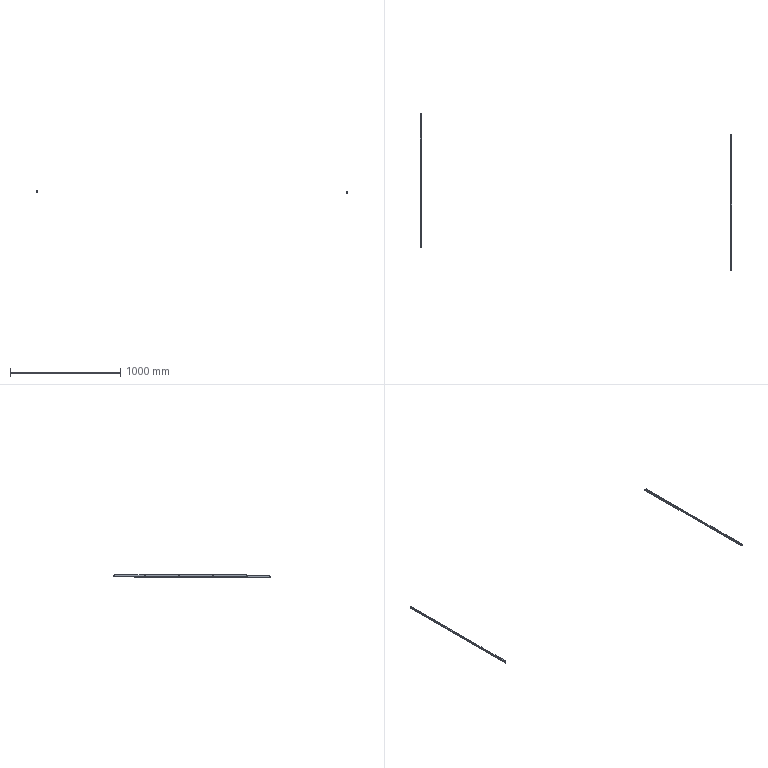NC program | NX | posted with a generic post | part box 2829 x 1430 x 20 mm
Whole program:
N10 G17 G21 G94 G90
(PLANAR_MILL_COPY_COPY_1 , TOOL : D16-48-D16-100-3T-FINISH)
N12 T01 M6
N14 G54
N16 G17 G0 G90 X623.5 Y0. B0. C0. S4000 M3
N18 G43 Z34. H1
N20 Z5.
N22 G94 G1 Z3. F1000.
N24 X610.5
N26 X-610.5
N28 X-623.5
N30 Z5.
N32 G0 Z34.
N34 X623.5
N36 Z4.
N38 G1 Z2.
N40 X610.5
N42 X-610.5
N44 X-623.5
N46 Z4.
N48 G0 Z34.
N50 X623.5
N52 Z3.
N54 G1 Z1.
N56 X610.5
N58 X-610.5
N60 X-623.5
N62 Z3.
N64 G0 Z34.
N66 X623.5
N68 Z2.1
N70 G1 Z0.1
N72 X610.5
N74 X-610.5
N76 X-623.5
N78 Z2.1
N80 G0 Z34.
(PLANAR_MILL_COPY_COPY_1_COPY , TOOL : D16-48-D16-100-3T-FINISH)
N82 X623.5
N84 Z2.
N86 G1 Z0.
N88 X610.5
N90 X-610.5
N92 X-623.5
N94 Z2.
N96 G0 Z34.
N98 M5
(PLANAR_MILL_2_COPY_1 , TOOL : D8-25-D8-60-3T-FINISH)
N100 T03 M6
N102 G54
N104 G17 G0 G90 X-606.4 Y11. B0. C0. S4500 M3
N106 G43 Z30. H3
N108 Z1.
N110 G94 G1 Z-1. F1200.
N112 Y5.
N114 Y-5.
N116 X-604.6
N118 Y5.
N120 Y11.
N122 Z1.
N124 G0 X-606.4 Z0.
N126 G1 Z-2.
N128 Y5.
N130 Y-5.
N132 X-604.6
N134 Y5.
N136 Y11.
N138 Z0.
N140 G0 X-606.4 Z-1.
N142 G1 Z-3.
N144 Y5.
N146 Y-5.
N148 X-604.6
N150 Y5.
N152 Y11.
N154 Z-1.
N156 G0 X-606.4 Z-2.
N158 G1 Z-4.
N160 Y5.
N162 Y-5.
N164 X-604.6
N166 Y5.
N168 Y11.
N170 Z-2.
N172 G0 X-606.4 Z-3.
N174 G1 Z-5.
N176 Y5.
N178 Y-5.
N180 X-604.6
N182 Y5.
N184 Y11.
N186 Z-3.
N188 G0 X-606.4 Z-4.
N190 G1 Z-6.
N192 Y5.
N194 Y-5.
N196 X-604.6
N198 Y5.
N200 Y11.
N202 Z-4.
N204 G0 X-606.4 Z-5.
N206 G1 Z-7.
N208 Y5.
N210 Y-5.
N212 X-604.6
N214 Y5.
N216 Y11.
N218 Z-5.
N220 G0 X-606.4 Z-5.9
N222 G1 Z-7.9
N224 Y5.
N226 Y-5.
N228 X-604.6
N230 Y5.
N232 Y11.
N234 Z-5.9
N236 G0 Z30.
N238 X-325.4
N240 Z1.
N242 G1 Z-1.
N244 Y5.
N246 Y-5.
N248 X-323.6
N250 Y5.
N252 Y11.
N254 Z1.
N256 G0 X-325.4 Z0.
N258 G1 Z-2.
N260 Y5.
N262 Y-5.
N264 X-323.6
N266 Y5.
N268 Y11.
N270 Z0.
N272 G0 X-325.4 Z-1.
N274 G1 Z-3.
N276 Y5.
N278 Y-5.
N280 X-323.6
N282 Y5.
N284 Y11.
N286 Z-1.
N288 G0 X-325.4 Z-2.
N290 G1 Z-4.
N292 Y5.
N294 Y-5.
N296 X-323.6
N298 Y5.
N300 Y11.
N302 Z-2.
N304 G0 X-325.4 Z-3.
N306 G1 Z-5.
N308 Y5.
N310 Y-5.
N312 X-323.6
N314 Y5.
N316 Y11.
N318 Z-3.
N320 G0 X-325.4 Z-4.
N322 G1 Z-6.
N324 Y5.
N326 Y-5.
N328 X-323.6
N330 Y5.
N332 Y11.
N334 Z-4.
N336 G0 X-325.4 Z-5.
N338 G1 Z-7.
N340 Y5.
N342 Y-5.
N344 X-323.6
N346 Y5.
N348 Y11.
N350 Z-5.
N352 G0 X-325.4 Z-5.9
N354 G1 Z-7.9
N356 Y5.
N358 Y-5.
N360 X-323.6
N362 Y5.
N364 Y11.
N366 Z-5.9
N368 G0 Z30.
N370 X-15.4
N372 Z1.
N374 G1 Z-1.
N376 Y5.
N378 Y-5.
N380 X-13.6
N382 Y5.
N384 Y11.
N386 Z1.
N388 G0 X-15.4 Z0.
N390 G1 Z-2.
N392 Y5.
N394 Y-5.
N396 X-13.6
N398 Y5.
N400 Y11.
N402 Z0.
N404 G0 X-15.4 Z-1.
N406 G1 Z-3.
N408 Y5.
N410 Y-5.
N412 X-13.6
N414 Y5.
N416 Y11.
N418 Z-1.
N420 G0 X-15.4 Z-2.
N422 G1 Z-4.
N424 Y5.
N426 Y-5.
N428 X-13.6
N430 Y5.
N432 Y11.
N434 Z-2.
N436 G0 X-15.4 Z-3.
N438 G1 Z-5.
N440 Y5.
N442 Y-5.
N444 X-13.6
N446 Y5.
N448 Y11.
N450 Z-3.
N452 G0 X-15.4 Z-4.
N454 G1 Z-6.
N456 Y5.
N458 Y-5.
N460 X-13.6
N462 Y5.
N464 Y11.
N466 Z-4.
N468 G0 X-15.4 Z-5.
N470 G1 Z-7.
N472 Y5.
N474 Y-5.
N476 X-13.6
N478 Y5.
N480 Y11.
N482 Z-5.
N484 G0 X-15.4 Z-5.9
N486 G1 Z-7.9
N488 Y5.
N490 Y-5.
N492 X-13.6
N494 Y5.
N496 Y11.
N498 Z-5.9
N500 G0 Z30.
N502 X294.6
N504 Z1.
N506 G1 Z-1.
N508 Y5.
N510 Y-5.
N512 X296.4
N514 Y5.
N516 Y11.
N518 Z1.
N520 G0 X294.6 Z0.
N522 G1 Z-2.
N524 Y5.
N526 Y-5.
N528 X296.4
N530 Y5.
N532 Y11.
N534 Z0.
N536 G0 X294.6 Z-1.
N538 G1 Z-3.
N540 Y5.
N542 Y-5.
N544 X296.4
N546 Y5.
N548 Y11.
N550 Z-1.
N552 G0 X294.6 Z-2.
N554 G1 Z-4.
N556 Y5.
N558 Y-5.
N560 X296.4
N562 Y5.
N564 Y11.
N566 Z-2.
N568 G0 X294.6 Z-3.
N570 G1 Z-5.
N572 Y5.
N574 Y-5.
N576 X296.4
N578 Y5.
N580 Y11.
N582 Z-3.
N584 G0 X294.6 Z-4.
N586 G1 Z-6.
N588 Y5.
N590 Y-5.
N592 X296.4
N594 Y5.
N596 Y11.
N598 Z-4.
N600 G0 X294.6 Z-5.
N602 G1 Z-7.
N604 Y5.
N606 Y-5.
N608 X296.4
N610 Y5.
N612 Y11.
N614 Z-5.
N616 G0 X294.6 Z-5.9
N618 G1 Z-7.9
N620 Y5.
N622 Y-5.
N624 X296.4
N626 Y5.
N628 Y11.
N630 Z-5.9
N632 G0 Z30.
N634 X604.6
N636 Z1.
N638 G1 Z-1.
N640 Y5.
N642 Y-5.
N644 X606.4
N646 Y5.
N648 Y11.
N650 Z1.
N652 G0 X604.6 Z0.
N654 G1 Z-2.
N656 Y5.
N658 Y-5.
N660 X606.4
N662 Y5.
N664 Y11.
N666 Z0.
N668 G0 X604.6 Z-1.
N670 G1 Z-3.
N672 Y5.
N674 Y-5.
N676 X606.4
N678 Y5.
N680 Y11.
N682 Z-1.
N684 G0 X604.6 Z-2.
N686 G1 Z-4.
N688 Y5.
N690 Y-5.
N692 X606.4
N694 Y5.
N696 Y11.
N698 Z-2.
N700 G0 X604.6 Z-3.
N702 G1 Z-5.
N704 Y5.
N706 Y-5.
N708 X606.4
N710 Y5.
N712 Y11.
N714 Z-3.
N716 G0 X604.6 Z-4.
N718 G1 Z-6.
N720 Y5.
N722 Y-5.
N724 X606.4
N726 Y5.
N728 Y11.
N730 Z-4.
N732 G0 X604.6 Z-5.
N734 G1 Z-7.
N736 Y5.
N738 Y-5.
N740 X606.4
N742 Y5.
N744 Y11.
N746 Z-5.
N748 G0 X604.6 Z-5.9
N750 G1 Z-7.9
N752 Y5.
N754 Y-5.
N756 X606.4
N758 Y5.
N760 Y11.
N762 Z-5.9
N764 G0 Z30.
(PLANAR_MILL_2_COPY_1_COPY , TOOL : D8-25-D8-60-3T-FINISH)
N766 X-606.326 Y11.985
N768 Z-6.
N770 G1 Z-8. F1000.
N772 G41 X-606.5 Y11. D3
N774 Y5.
N776 Y-5.
N778 X-604.5
N780 Y5.
N782 Y11.
N784 G40
N786 X-604.674 Y11.985
N788 Z-6.
N790 G0 Z30.
N792 X-325.326
N794 Z-6.
N796 G1 Z-8.
N798 G41 X-325.5 Y11.
N800 Y5.
N802 Y-5.
N804 X-323.5
N806 Y5.
N808 Y11.
N810 G40
N812 X-323.674 Y11.985
N814 Z-6.
N816 G0 Z30.
N818 X-15.326
N820 Z-6.
N822 G1 Z-8.
N824 G41 X-15.5 Y11.
N826 Y5.
N828 Y-5.
N830 X-13.5
N832 Y5.
N834 Y11.
N836 G40
N838 X-13.674 Y11.985
N840 Z-6.
N842 G0 Z30.
N844 X294.674
N846 Z-6.
N848 G1 Z-8.
N850 G41 X294.5 Y11.
N852 Y5.
N854 Y-5.
N856 X296.5
N858 Y5.
N860 Y11.
N862 G40
N864 X296.326 Y11.985
N866 Z-6.
N868 G0 Z30.
N870 X604.674
N872 Z-6.
N874 G1 Z-8.
N876 G41 X604.5 Y11.
N878 Y5.
N880 Y-5.
N882 X606.5
N884 Y5.
N886 Y11.
N888 G40
N890 X606.326 Y11.985
N892 Z-6.
N894 G0 Z30.
N896 M5
(PLANAR_MILL_3_COPY , TOOL : 倒角D6-90度)
N898 T04 M6
N900 G54
N902 G17 G0 G90 X452.5 Y-8.5 B0. C0. S3000 M3
N904 G43 Z30. H4
N906 Z0.5
N908 G94 G1 Z-1.5 F1000.
N910 G3 X450.5 Y-6.5 R2.
N912 G1 X300.5
N914 G2 X299. Y-5. R1.5
N916 G1 Y5.
N918 G2 X300.5 Y6.5 R1.5
N920 G1 X600.5
N922 G2 X602. Y5. R1.5
N924 G1 Y-5.
N926 G2 X600.5 Y-6.5 R1.5
N928 G1 X450.5
N930 G3 X448.5 Y-8.5 R2.
N932 G1 Z0.5
N934 G0 Z30.
N936 X142.5
N938 Z0.5
N940 G1 Z-1.5
N942 G3 X140.5 Y-6.5 R2.
N944 G1 X-9.5
N946 G2 X-11. Y-5. R1.5
N948 G1 Y5.
N950 G2 X-9.5 Y6.5 R1.5
N952 G1 X290.5
N954 G2 X292. Y5. R1.5
N956 G1 Y-5.
N958 G2 X290.5 Y-6.5 R1.5
N960 G1 X140.5
N962 G3 X138.5 Y-8.5 R2.
N964 G1 Z0.5
N966 G0 Z30.
N968 X-167.5
N970 Z0.5
N972 G1 Z-1.5
N974 G3 X-169.5 Y-6.5 R2.
N976 G1 X-319.5
N978 G2 X-321. Y-5. R1.5
N980 G1 Y5.
N982 G2 X-319.5 Y6.5 R1.5
N984 G1 X-19.5
N986 G2 X-18. Y5. R1.5
N988 G1 Y-5.
N990 G2 X-19.5 Y-6.5 R1.5
N992 G1 X-169.5
N994 G3 X-171.5 Y-8.5 R2.
N996 G1 Z0.5
N998 G0 Z30.
N1000 X-467. Y8.5
N1002 Z0.5
N1004 G1 Z-1.5
N1006 G3 X-465. Y6.5 R2.
N1008 G1 X-329.5
N1010 G2 X-328. Y5. R1.5
N1012 G1 Y-5.
N1014 G2 X-329.5 Y-6.5 R1.5
N1016 G1 X-600.5
N1018 G2 X-602. Y-5. R1.5
N1020 G1 Y5.
N1022 G2 X-600.5 Y6.5 R1.5
N1024 G1 X-465.
N1026 G3 X-463. Y8.5 R2.
N1028 G1 Z0.5
N1030 G0 Z30.
N1032 M5
N1034 M2